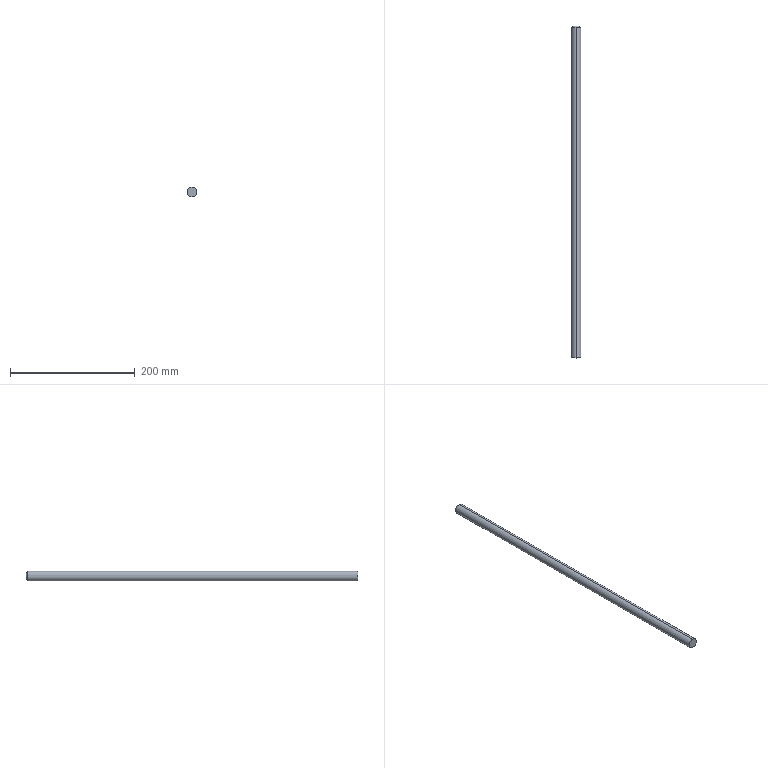Part | SolidWorks | features Chamfer 1, Extrusion 1 | 1 solid | 6 faces | box 16 x 531.5 x 16 mm | volume 106666 mm3 | cone 2 | cylinder 2 | plane 2 | commonest cylinder face diameters 16 x2
STEP:
#1=CARTESIAN_POINT('',(0.,531.5,5.));
#2=VERTEX_POINT('',#1);
#3=CARTESIAN_POINT('',(0.,531.5,-5.));
#4=VERTEX_POINT('',#3);
#5=CARTESIAN_POINT('',(0.,531.5,0.));
#6=DIRECTION('',(0.,1.,0.));
#7=DIRECTION('',(0.,0.,1.));
#8=AXIS2_PLACEMENT_3D('',#5,#6,#7);
#9=CIRCLE('',#8,5.);
#10=EDGE_CURVE('',#2,#4,#9,.T.);
#11=ORIENTED_EDGE('',*,*,#10,.F.);
#12=CARTESIAN_POINT('',(0.,528.5,8.));
#13=VERTEX_POINT('',#12);
#14=CARTESIAN_POINT('',(0.,531.5,5.));
#15=DIRECTION('',(0.,-0.7071,0.7071));
#16=VECTOR('',#15,1000.);
#17=LINE('',#14,#16);
#18=EDGE_CURVE('',#2,#13,#17,.T.);
#19=ORIENTED_EDGE('',*,*,#18,.T.);
#20=CARTESIAN_POINT('',(0.,528.5,-8.));
#21=VERTEX_POINT('',#20);
#22=CARTESIAN_POINT('',(0.,528.5,0.));
#23=DIRECTION('',(0.,-1.,0.));
#24=DIRECTION('',(0.,0.,1.));
#25=AXIS2_PLACEMENT_3D('',#22,#23,#24);
#26=CIRCLE('',#25,8.);
#27=EDGE_CURVE('',#21,#13,#26,.T.);
#28=ORIENTED_EDGE('',*,*,#27,.F.);
#29=CARTESIAN_POINT('',(0.,531.5,-5.));
#30=DIRECTION('',(0.,-0.7071,-0.7071));
#31=VECTOR('',#30,1000.);
#32=LINE('',#29,#31);
#33=EDGE_CURVE('',#4,#21,#32,.T.);
#34=ORIENTED_EDGE('',*,*,#33,.F.);
#35=EDGE_LOOP('',(#11,#19,#28,#34));
#36=FACE_OUTER_BOUND('',#35,.T.);
#37=CARTESIAN_POINT('',(0.,531.5,0.));
#38=DIRECTION('',(0.,-1.,0.));
#39=DIRECTION('',(0.,0.,-1.));
#40=AXIS2_PLACEMENT_3D('',#37,#38,#39);
#41=CONICAL_SURFACE('',#40,5.,0.7854);
#42=ADVANCED_FACE('',(#36),#41,.T.);
#43=ORIENTED_EDGE('',*,*,#27,.T.);
#44=CARTESIAN_POINT('',(0.,0.,8.));
#45=VERTEX_POINT('',#44);
#46=CARTESIAN_POINT('',(0.,531.5,8.));
#47=DIRECTION('',(0.,-1.,0.));
#48=VECTOR('',#47,1000.);
#49=LINE('',#46,#48);
#50=EDGE_CURVE('',#13,#45,#49,.T.);
#51=ORIENTED_EDGE('',*,*,#50,.T.);
#52=CARTESIAN_POINT('',(0.,0.,-8.));
#53=VERTEX_POINT('',#52);
#54=CARTESIAN_POINT('',(0.,0.,0.));
#55=DIRECTION('',(0.,1.,0.));
#56=DIRECTION('',(0.,0.,1.));
#57=AXIS2_PLACEMENT_3D('',#54,#55,#56);
#58=CIRCLE('',#57,8.);
#59=EDGE_CURVE('',#45,#53,#58,.T.);
#60=ORIENTED_EDGE('',*,*,#59,.T.);
#61=CARTESIAN_POINT('',(0.,531.5,-8.));
#62=DIRECTION('',(0.,-1.,0.));
#63=VECTOR('',#62,1000.);
#64=LINE('',#61,#63);
#65=EDGE_CURVE('',#21,#53,#64,.T.);
#66=ORIENTED_EDGE('',*,*,#65,.F.);
#67=EDGE_LOOP('',(#43,#51,#60,#66));
#68=FACE_OUTER_BOUND('',#67,.T.);
#69=CARTESIAN_POINT('',(0.,531.5,0.));
#70=DIRECTION('',(0.,-1.,0.));
#71=DIRECTION('',(0.,0.,-1.));
#72=AXIS2_PLACEMENT_3D('',#69,#70,#71);
#73=CYLINDRICAL_SURFACE('',#72,8.);
#74=ADVANCED_FACE('',(#68),#73,.T.);
#75=ORIENTED_EDGE('',*,*,#50,.F.);
#76=CARTESIAN_POINT('',(0.,528.5,0.));
#77=DIRECTION('',(0.,-1.,0.));
#78=DIRECTION('',(0.,0.,1.));
#79=AXIS2_PLACEMENT_3D('',#76,#77,#78);
#80=CIRCLE('',#79,8.);
#81=EDGE_CURVE('',#13,#21,#80,.T.);
#82=ORIENTED_EDGE('',*,*,#81,.T.);
#83=ORIENTED_EDGE('',*,*,#65,.T.);
#84=CARTESIAN_POINT('',(0.,0.,0.));
#85=DIRECTION('',(0.,1.,0.));
#86=DIRECTION('',(0.,0.,1.));
#87=AXIS2_PLACEMENT_3D('',#84,#85,#86);
#88=CIRCLE('',#87,8.);
#89=EDGE_CURVE('',#53,#45,#88,.T.);
#90=ORIENTED_EDGE('',*,*,#89,.T.);
#91=EDGE_LOOP('',(#75,#82,#83,#90));
#92=FACE_OUTER_BOUND('',#91,.T.);
#93=CARTESIAN_POINT('',(0.,531.5,0.));
#94=DIRECTION('',(0.,-1.,0.));
#95=DIRECTION('',(0.,0.,-1.));
#96=AXIS2_PLACEMENT_3D('',#93,#94,#95);
#97=CYLINDRICAL_SURFACE('',#96,8.);
#98=ADVANCED_FACE('',(#92),#97,.T.);
#99=CARTESIAN_POINT('',(0.,531.5,0.));
#100=DIRECTION('',(0.,1.,0.));
#101=DIRECTION('',(0.,0.,1.));
#102=AXIS2_PLACEMENT_3D('',#99,#100,#101);
#103=CIRCLE('',#102,5.);
#104=EDGE_CURVE('',#4,#2,#103,.T.);
#105=ORIENTED_EDGE('',*,*,#104,.T.);
#106=ORIENTED_EDGE('',*,*,#10,.T.);
#107=EDGE_LOOP('',(#105,#106));
#108=FACE_OUTER_BOUND('',#107,.T.);
#109=CARTESIAN_POINT('',(0.,531.5,0.));
#110=DIRECTION('',(0.,1.,0.));
#111=DIRECTION('',(0.,0.,1.));
#112=AXIS2_PLACEMENT_3D('',#109,#110,#111);
#113=PLANE('',#112);
#114=ADVANCED_FACE('',(#108),#113,.T.);
#115=ORIENTED_EDGE('',*,*,#89,.F.);
#116=ORIENTED_EDGE('',*,*,#59,.F.);
#117=EDGE_LOOP('',(#115,#116));
#118=FACE_OUTER_BOUND('',#117,.T.);
#119=CARTESIAN_POINT('',(0.,0.,0.));
#120=DIRECTION('',(0.,1.,0.));
#121=DIRECTION('',(0.,0.,1.));
#122=AXIS2_PLACEMENT_3D('',#119,#120,#121);
#123=PLANE('',#122);
#124=ADVANCED_FACE('',(#118),#123,.F.);
#125=ORIENTED_EDGE('',*,*,#18,.F.);
#126=ORIENTED_EDGE('',*,*,#104,.F.);
#127=ORIENTED_EDGE('',*,*,#33,.T.);
#128=ORIENTED_EDGE('',*,*,#81,.F.);
#129=EDGE_LOOP('',(#125,#126,#127,#128));
#130=FACE_OUTER_BOUND('',#129,.T.);
#131=CARTESIAN_POINT('',(0.,531.5,0.));
#132=DIRECTION('',(0.,-1.,0.));
#133=DIRECTION('',(0.,0.,-1.));
#134=AXIS2_PLACEMENT_3D('',#131,#132,#133);
#135=CONICAL_SURFACE('',#134,5.,0.7854);
#136=ADVANCED_FACE('',(#130),#135,.T.);
#137=CLOSED_SHELL('',(#42,#74,#98,#114,#124,#136));
#138=MANIFOLD_SOLID_BREP('',#137);
#139=CARTESIAN_POINT('',(0.,0.,0.));
#140=DIRECTION('',(0.,0.,1.));
#141=DIRECTION('',(1.,0.,0.));
#142=AXIS2_PLACEMENT_3D('',#139,#140,#141);
#143=(LENGTH_UNIT()NAMED_UNIT(*)SI_UNIT(.MILLI.,.METRE.));
#144=UNCERTAINTY_MEASURE_WITH_UNIT(LENGTH_MEASURE(0.00001),#143,'','');
#145=(NAMED_UNIT(*)PLANE_ANGLE_UNIT()SI_UNIT($,.RADIAN.));
#146=(NAMED_UNIT(*)SI_UNIT($,.STERADIAN.)SOLID_ANGLE_UNIT());
#147=(GEOMETRIC_REPRESENTATION_CONTEXT(3)GLOBAL_UNCERTAINTY_ASSIGNED_CONTEXT((#144))GLOBAL_UNIT_ASSIGNED_CONTEXT((#143,#145,#146))REPRESENTATION_CONTEXT('',''));
#148=ADVANCED_BREP_SHAPE_REPRESENTATION('',(#138,#142),#147);